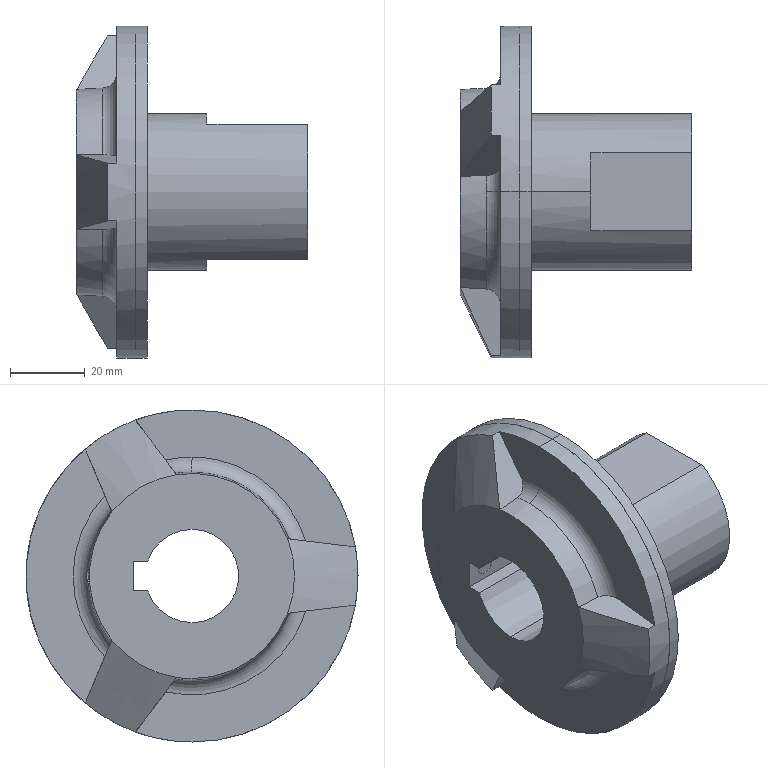Part | STEP file | TL350_2_25JHub | 1 solid | 56 faces | box 62 x 89 x 89 mm | volume 108806 mm3 | plane 30 | cylinder 15 | cone 7 | torus 4 | commonest cylinder face diameters 4.917 x4 89 x4 25 x3 42 x2 88 x2